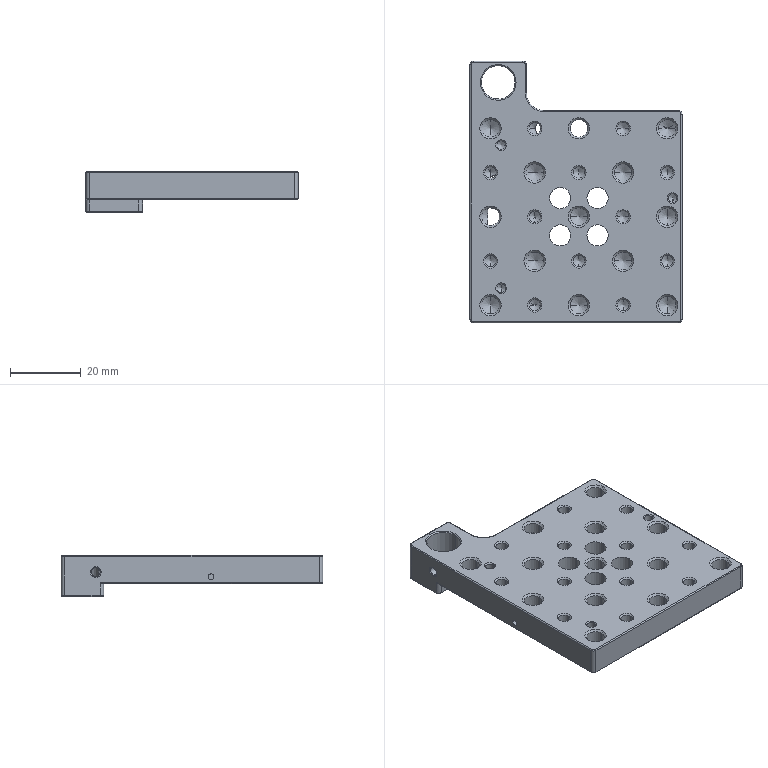Part | STEP file | 1 solid | 281 faces | box 60 x 74 x 11.6 mm | volume 26262 mm3 | cylinder 125 | cone 116 | plane 26 | torus 14 | commonest cylinder face diameters 5 x26 3.3 x24 6 x21 1.6 x20 0.6 x14 2.5 x8